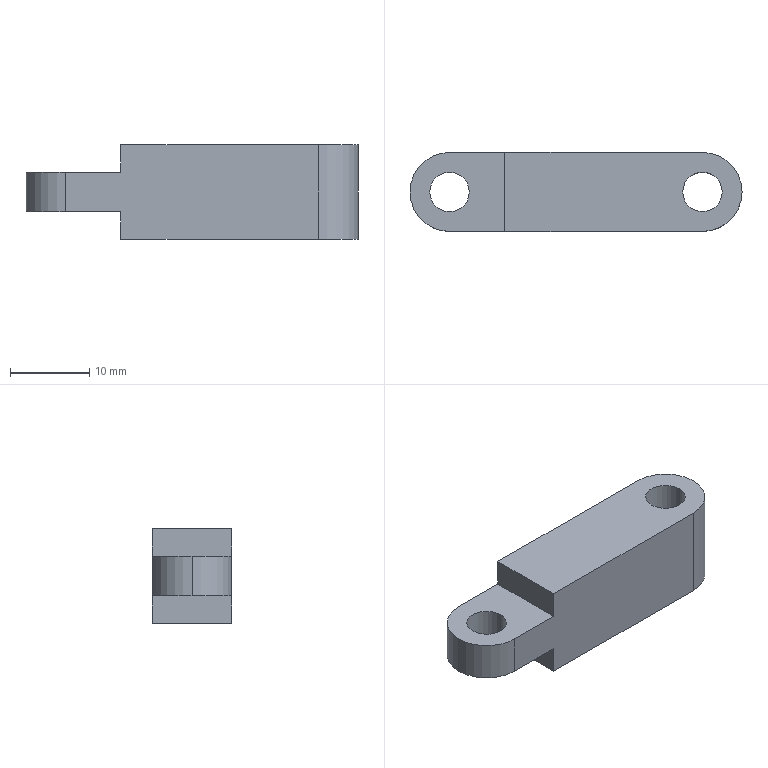Part | STEP file | gripper arm 1_default | 1 solid | 16 faces | box 42 x 10 x 12 mm | volume 3684 mm3 | cylinder 8 | plane 8 | commonest cylinder face diameters 5 x4 10 x4
STEP:
#1=CARTESIAN_POINT('',(0.,0.,0.));
#2=DIRECTION('',(0.,0.,1.));
#3=DIRECTION('',(1.,0.,0.));
#4=AXIS2_PLACEMENT_3D('',#1,#2,#3);
#5=CARTESIAN_POINT('',(18.5,0.,0.));
#6=VERTEX_POINT('',#5);
#7=CARTESIAN_POINT('',(18.5,0.,12.));
#8=VERTEX_POINT('',#7);
#9=CARTESIAN_POINT('',(18.5,0.,0.));
#10=DIRECTION('',(0.,0.,1.));
#11=VECTOR('',#10,1.);
#12=LINE('',#9,#11);
#13=CARTESIAN_POINT('',(16.,0.,0.));
#14=DIRECTION('',(0.,0.,1.));
#15=DIRECTION('',(1.,0.,0.));
#16=AXIS2_PLACEMENT_3D('',#13,#14,#15);
#17=CYLINDRICAL_SURFACE('',#16,2.5);
#18=CARTESIAN_POINT('',(6.283,0.));
#19=DIRECTION('',(0.,1.));
#20=VECTOR('',#19,1.);
#21=LINE('',#18,#20);
#22=(GEOMETRIC_REPRESENTATION_CONTEXT(2)PARAMETRIC_REPRESENTATION_CONTEXT()REPRESENTATION_CONTEXT('',''));
#23=DEFINITIONAL_REPRESENTATION('',(#21),#22);
#24=PCURVE('',#17,#23);
#25=CARTESIAN_POINT('',(16.,0.,0.));
#26=DIRECTION('',(0.,0.,1.));
#27=DIRECTION('',(1.,0.,0.));
#28=AXIS2_PLACEMENT_3D('',#25,#26,#27);
#29=CYLINDRICAL_SURFACE('',#28,2.5);
#30=CARTESIAN_POINT('',(0.,0.));
#31=DIRECTION('',(0.,1.));
#32=VECTOR('',#31,1.);
#33=LINE('',#30,#32);
#34=(GEOMETRIC_REPRESENTATION_CONTEXT(2)PARAMETRIC_REPRESENTATION_CONTEXT()REPRESENTATION_CONTEXT('',''));
#35=DEFINITIONAL_REPRESENTATION('',(#33),#34);
#36=PCURVE('',#29,#35);
#37=SURFACE_CURVE('',#12,(#24,#36),.PCURVE_S1.);
#38=EDGE_CURVE('',#6,#8,#37,.T.);
#39=ORIENTED_EDGE('',*,*,#38,.T.);
#40=CARTESIAN_POINT('',(13.5,0.,12.));
#41=VERTEX_POINT('',#40);
#42=CARTESIAN_POINT('',(16.,0.,12.));
#43=DIRECTION('',(0.,0.,1.));
#44=DIRECTION('',(1.,0.,0.));
#45=AXIS2_PLACEMENT_3D('',#42,#43,#44);
#46=CIRCLE('',#45,2.5);
#47=CARTESIAN_POINT('',(0.,12.));
#48=DIRECTION('',(1.,0.));
#49=VECTOR('',#48,1.);
#50=LINE('',#47,#49);
#51=(GEOMETRIC_REPRESENTATION_CONTEXT(2)PARAMETRIC_REPRESENTATION_CONTEXT()REPRESENTATION_CONTEXT('',''));
#52=DEFINITIONAL_REPRESENTATION('',(#50),#51);
#53=PCURVE('',#17,#52);
#54=CARTESIAN_POINT('',(0.,0.,12.));
#55=DIRECTION('',(0.,0.,1.));
#56=DIRECTION('',(1.,0.,0.));
#57=AXIS2_PLACEMENT_3D('',#54,#55,#56);
#58=PLANE('',#57);
#59=CARTESIAN_POINT('',(16.,0.));
#60=DIRECTION('',(1.,0.));
#61=AXIS2_PLACEMENT_2D('',#59,#60);
#62=CIRCLE('',#61,2.5);
#63=(GEOMETRIC_REPRESENTATION_CONTEXT(2)PARAMETRIC_REPRESENTATION_CONTEXT()REPRESENTATION_CONTEXT('',''));
#64=DEFINITIONAL_REPRESENTATION('',(#62),#63);
#65=PCURVE('',#58,#64);
#66=SURFACE_CURVE('',#46,(#53,#65),.PCURVE_S1.);
#67=EDGE_CURVE('',#41,#8,#66,.T.);
#68=ORIENTED_EDGE('',*,*,#67,.F.);
#69=CARTESIAN_POINT('',(13.5,0.,0.));
#70=VERTEX_POINT('',#69);
#71=CARTESIAN_POINT('',(13.5,0.,0.));
#72=DIRECTION('',(0.,0.,1.));
#73=VECTOR('',#72,1.);
#74=LINE('',#71,#73);
#75=CARTESIAN_POINT('',(3.142,0.));
#76=DIRECTION('',(0.,1.));
#77=VECTOR('',#76,1.);
#78=LINE('',#75,#77);
#79=(GEOMETRIC_REPRESENTATION_CONTEXT(2)PARAMETRIC_REPRESENTATION_CONTEXT()REPRESENTATION_CONTEXT('',''));
#80=DEFINITIONAL_REPRESENTATION('',(#78),#79);
#81=PCURVE('',#17,#80);
#82=CARTESIAN_POINT('',(3.142,0.));
#83=DIRECTION('',(0.,1.));
#84=VECTOR('',#83,1.);
#85=LINE('',#82,#84);
#86=(GEOMETRIC_REPRESENTATION_CONTEXT(2)PARAMETRIC_REPRESENTATION_CONTEXT()REPRESENTATION_CONTEXT('',''));
#87=DEFINITIONAL_REPRESENTATION('',(#85),#86);
#88=PCURVE('',#29,#87);
#89=SURFACE_CURVE('',#74,(#81,#88),.PCURVE_S1.);
#90=EDGE_CURVE('',#70,#41,#89,.T.);
#91=ORIENTED_EDGE('',*,*,#90,.F.);
#92=CARTESIAN_POINT('',(16.,0.,0.));
#93=DIRECTION('',(0.,0.,1.));
#94=DIRECTION('',(1.,0.,0.));
#95=AXIS2_PLACEMENT_3D('',#92,#93,#94);
#96=CIRCLE('',#95,2.5);
#97=CARTESIAN_POINT('',(0.,0.));
#98=DIRECTION('',(1.,0.));
#99=VECTOR('',#98,1.);
#100=LINE('',#97,#99);
#101=(GEOMETRIC_REPRESENTATION_CONTEXT(2)PARAMETRIC_REPRESENTATION_CONTEXT()REPRESENTATION_CONTEXT('',''));
#102=DEFINITIONAL_REPRESENTATION('',(#100),#101);
#103=PCURVE('',#17,#102);
#104=CARTESIAN_POINT('',(0.,0.,0.));
#105=DIRECTION('',(0.,0.,1.));
#106=DIRECTION('',(1.,0.,0.));
#107=AXIS2_PLACEMENT_3D('',#104,#105,#106);
#108=PLANE('',#107);
#109=CARTESIAN_POINT('',(16.,0.));
#110=DIRECTION('',(1.,0.));
#111=AXIS2_PLACEMENT_2D('',#109,#110);
#112=CIRCLE('',#111,2.5);
#113=(GEOMETRIC_REPRESENTATION_CONTEXT(2)PARAMETRIC_REPRESENTATION_CONTEXT()REPRESENTATION_CONTEXT('',''));
#114=DEFINITIONAL_REPRESENTATION('',(#112),#113);
#115=PCURVE('',#108,#114);
#116=SURFACE_CURVE('',#96,(#103,#115),.PCURVE_S1.);
#117=EDGE_CURVE('',#70,#6,#116,.T.);
#118=ORIENTED_EDGE('',*,*,#117,.T.);
#119=EDGE_LOOP('',(#39,#68,#91,#118));
#120=FACE_BOUND('',#119,.F.);
#121=ADVANCED_FACE('',(#120),#17,.F.);
#122=CARTESIAN_POINT('',(-13.5,0.,3.5));
#123=VERTEX_POINT('',#122);
#124=CARTESIAN_POINT('',(-13.5,0.,8.5));
#125=VERTEX_POINT('',#124);
#126=CARTESIAN_POINT('',(-13.5,0.,0.));
#127=DIRECTION('',(0.,0.,1.));
#128=VECTOR('',#127,1.);
#129=LINE('',#126,#128);
#130=CARTESIAN_POINT('',(-16.,0.,0.));
#131=DIRECTION('',(0.,0.,1.));
#132=DIRECTION('',(1.,0.,0.));
#133=AXIS2_PLACEMENT_3D('',#130,#131,#132);
#134=CYLINDRICAL_SURFACE('',#133,2.5);
#135=CARTESIAN_POINT('',(6.283,0.));
#136=DIRECTION('',(0.,1.));
#137=VECTOR('',#136,1.);
#138=LINE('',#135,#137);
#139=(GEOMETRIC_REPRESENTATION_CONTEXT(2)PARAMETRIC_REPRESENTATION_CONTEXT()REPRESENTATION_CONTEXT('',''));
#140=DEFINITIONAL_REPRESENTATION('',(#138),#139);
#141=PCURVE('',#134,#140);
#142=CARTESIAN_POINT('',(-16.,0.,0.));
#143=DIRECTION('',(0.,0.,1.));
#144=DIRECTION('',(1.,0.,0.));
#145=AXIS2_PLACEMENT_3D('',#142,#143,#144);
#146=CYLINDRICAL_SURFACE('',#145,2.5);
#147=CARTESIAN_POINT('',(0.,0.));
#148=DIRECTION('',(0.,1.));
#149=VECTOR('',#148,1.);
#150=LINE('',#147,#149);
#151=(GEOMETRIC_REPRESENTATION_CONTEXT(2)PARAMETRIC_REPRESENTATION_CONTEXT()REPRESENTATION_CONTEXT('',''));
#152=DEFINITIONAL_REPRESENTATION('',(#150),#151);
#153=PCURVE('',#146,#152);
#154=SURFACE_CURVE('',#129,(#141,#153),.PCURVE_S1.);
#155=EDGE_CURVE('',#123,#125,#154,.T.);
#156=ORIENTED_EDGE('',*,*,#155,.T.);
#157=CARTESIAN_POINT('',(-18.5,0.,8.5));
#158=VERTEX_POINT('',#157);
#159=CARTESIAN_POINT('',(-16.,0.,8.5));
#160=DIRECTION('',(0.,0.,-1.));
#161=DIRECTION('',(1.,0.,0.));
#162=AXIS2_PLACEMENT_3D('',#159,#160,#161);
#163=CIRCLE('',#162,2.5);
#164=CARTESIAN_POINT('',(6.283,8.5));
#165=DIRECTION('',(-1.,0.));
#166=VECTOR('',#165,1.);
#167=LINE('',#164,#166);
#168=(GEOMETRIC_REPRESENTATION_CONTEXT(2)PARAMETRIC_REPRESENTATION_CONTEXT()REPRESENTATION_CONTEXT('',''));
#169=DEFINITIONAL_REPRESENTATION('',(#167),#168);
#170=PCURVE('',#134,#169);
#171=CARTESIAN_POINT('',(0.,0.,8.5));
#172=DIRECTION('',(0.,0.,1.));
#173=DIRECTION('',(1.,0.,0.));
#174=AXIS2_PLACEMENT_3D('',#171,#172,#173);
#175=PLANE('',#174);
#176=CARTESIAN_POINT('',(-13.5,0.));
#177=CARTESIAN_POINT('',(-13.5,-4.33));
#178=CARTESIAN_POINT('',(-17.25,-2.165));
#179=CARTESIAN_POINT('',(-21.,0.));
#180=CARTESIAN_POINT('',(-17.25,2.165));
#181=CARTESIAN_POINT('',(-13.5,4.33));
#182=CARTESIAN_POINT('',(-13.5,0.));
#183=(BOUNDED_CURVE()B_SPLINE_CURVE(2,(#176,#177,#178,#179,#180,#181,#182),.UNSPECIFIED.,.T.,.F.)B_SPLINE_CURVE_WITH_KNOTS((1,2,2,2,2,1),(-2.094,0.,2.094,4.189,6.283,8.378),.UNSPECIFIED.)CURVE()GEOMETRIC_REPRESENTATION_ITEM()RATIONAL_B_SPLINE_CURVE((1.,0.5,1.,0.5,1.,0.5,1.))REPRESENTATION_ITEM(''));
#184=(GEOMETRIC_REPRESENTATION_CONTEXT(2)PARAMETRIC_REPRESENTATION_CONTEXT()REPRESENTATION_CONTEXT('',''));
#185=DEFINITIONAL_REPRESENTATION('',(#183),#184);
#186=PCURVE('',#175,#185);
#187=SURFACE_CURVE('',#163,(#170,#186),.PCURVE_S1.);
#188=EDGE_CURVE('',#125,#158,#187,.T.);
#189=ORIENTED_EDGE('',*,*,#188,.T.);
#190=CARTESIAN_POINT('',(-18.5,0.,3.5));
#191=VERTEX_POINT('',#190);
#192=CARTESIAN_POINT('',(-18.5,0.,0.));
#193=DIRECTION('',(0.,0.,1.));
#194=VECTOR('',#193,1.);
#195=LINE('',#192,#194);
#196=CARTESIAN_POINT('',(3.142,0.));
#197=DIRECTION('',(0.,1.));
#198=VECTOR('',#197,1.);
#199=LINE('',#196,#198);
#200=(GEOMETRIC_REPRESENTATION_CONTEXT(2)PARAMETRIC_REPRESENTATION_CONTEXT()REPRESENTATION_CONTEXT('',''));
#201=DEFINITIONAL_REPRESENTATION('',(#199),#200);
#202=PCURVE('',#134,#201);
#203=CARTESIAN_POINT('',(3.142,0.));
#204=DIRECTION('',(0.,1.));
#205=VECTOR('',#204,1.);
#206=LINE('',#203,#205);
#207=(GEOMETRIC_REPRESENTATION_CONTEXT(2)PARAMETRIC_REPRESENTATION_CONTEXT()REPRESENTATION_CONTEXT('',''));
#208=DEFINITIONAL_REPRESENTATION('',(#206),#207);
#209=PCURVE('',#146,#208);
#210=SURFACE_CURVE('',#195,(#202,#209),.PCURVE_S1.);
#211=EDGE_CURVE('',#191,#158,#210,.T.);
#212=ORIENTED_EDGE('',*,*,#211,.F.);
#213=CARTESIAN_POINT('',(-16.,0.,3.5));
#214=DIRECTION('',(0.,0.,1.));
#215=DIRECTION('',(-1.,0.,0.));
#216=AXIS2_PLACEMENT_3D('',#213,#214,#215);
#217=CIRCLE('',#216,2.5);
#218=CARTESIAN_POINT('',(3.142,3.5));
#219=DIRECTION('',(1.,0.));
#220=VECTOR('',#219,1.);
#221=LINE('',#218,#220);
#222=(GEOMETRIC_REPRESENTATION_CONTEXT(2)PARAMETRIC_REPRESENTATION_CONTEXT()REPRESENTATION_CONTEXT('',''));
#223=DEFINITIONAL_REPRESENTATION('',(#221),#222);
#224=PCURVE('',#134,#223);
#225=CARTESIAN_POINT('',(0.,0.,3.5));
#226=DIRECTION('',(0.,0.,-1.));
#227=DIRECTION('',(-1.,0.,0.));
#228=AXIS2_PLACEMENT_3D('',#225,#226,#227);
#229=PLANE('',#228);
#230=CARTESIAN_POINT('',(18.5,0.));
#231=CARTESIAN_POINT('',(18.5,-4.33));
#232=CARTESIAN_POINT('',(14.75,-2.165));
#233=CARTESIAN_POINT('',(11.,0.));
#234=CARTESIAN_POINT('',(14.75,2.165));
#235=CARTESIAN_POINT('',(18.5,4.33));
#236=CARTESIAN_POINT('',(18.5,0.));
#237=(BOUNDED_CURVE()B_SPLINE_CURVE(2,(#230,#231,#232,#233,#234,#235,#236),.UNSPECIFIED.,.T.,.F.)B_SPLINE_CURVE_WITH_KNOTS((1,2,2,2,2,1),(-2.094,0.,2.094,4.189,6.283,8.378),.UNSPECIFIED.)CURVE()GEOMETRIC_REPRESENTATION_ITEM()RATIONAL_B_SPLINE_CURVE((1.,0.5,1.,0.5,1.,0.5,1.))REPRESENTATION_ITEM(''));
#238=(GEOMETRIC_REPRESENTATION_CONTEXT(2)PARAMETRIC_REPRESENTATION_CONTEXT()REPRESENTATION_CONTEXT('',''));
#239=DEFINITIONAL_REPRESENTATION('',(#237),#238);
#240=PCURVE('',#229,#239);
#241=SURFACE_CURVE('',#217,(#224,#240),.PCURVE_S1.);
#242=EDGE_CURVE('',#191,#123,#241,.T.);
#243=ORIENTED_EDGE('',*,*,#242,.T.);
#244=EDGE_LOOP('',(#156,#189,#212,#243));
#245=FACE_BOUND('',#244,.F.);
#246=ADVANCED_FACE('',(#245),#134,.F.);
#247=CARTESIAN_POINT('',(-16.,0.,8.5));
#248=DIRECTION('',(0.,0.,-1.));
#249=DIRECTION('',(1.,0.,0.));
#250=AXIS2_PLACEMENT_3D('',#247,#248,#249);
#251=CIRCLE('',#250,2.5);
#252=CARTESIAN_POINT('',(6.283,8.5));
#253=DIRECTION('',(-1.,0.));
#254=VECTOR('',#253,1.);
#255=LINE('',#252,#254);
#256=(GEOMETRIC_REPRESENTATION_CONTEXT(2)PARAMETRIC_REPRESENTATION_CONTEXT()REPRESENTATION_CONTEXT('',''));
#257=DEFINITIONAL_REPRESENTATION('',(#255),#256);
#258=PCURVE('',#146,#257);
#259=CARTESIAN_POINT('',(-13.5,0.));
#260=CARTESIAN_POINT('',(-13.5,-4.33));
#261=CARTESIAN_POINT('',(-17.25,-2.165));
#262=CARTESIAN_POINT('',(-21.,0.));
#263=CARTESIAN_POINT('',(-17.25,2.165));
#264=CARTESIAN_POINT('',(-13.5,4.33));
#265=CARTESIAN_POINT('',(-13.5,0.));
#266=(BOUNDED_CURVE()B_SPLINE_CURVE(2,(#259,#260,#261,#262,#263,#264,#265),.UNSPECIFIED.,.T.,.F.)B_SPLINE_CURVE_WITH_KNOTS((1,2,2,2,2,1),(-2.094,0.,2.094,4.189,6.283,8.378),.UNSPECIFIED.)CURVE()GEOMETRIC_REPRESENTATION_ITEM()RATIONAL_B_SPLINE_CURVE((1.,0.5,1.,0.5,1.,0.5,1.))REPRESENTATION_ITEM(''));
#267=(GEOMETRIC_REPRESENTATION_CONTEXT(2)PARAMETRIC_REPRESENTATION_CONTEXT()REPRESENTATION_CONTEXT('',''));
#268=DEFINITIONAL_REPRESENTATION('',(#266),#267);
#269=PCURVE('',#175,#268);
#270=SURFACE_CURVE('',#251,(#258,#269),.PCURVE_S1.);
#271=EDGE_CURVE('',#158,#125,#270,.T.);
#272=ORIENTED_EDGE('',*,*,#271,.T.);
#273=ORIENTED_EDGE('',*,*,#155,.F.);
#274=CARTESIAN_POINT('',(-16.,0.,3.5));
#275=DIRECTION('',(0.,0.,1.));
#276=DIRECTION('',(-1.,0.,0.));
#277=AXIS2_PLACEMENT_3D('',#274,#275,#276);
#278=CIRCLE('',#277,2.5);
#279=CARTESIAN_POINT('',(-3.142,3.5));
#280=DIRECTION('',(1.,0.));
#281=VECTOR('',#280,1.);
#282=LINE('',#279,#281);
#283=(GEOMETRIC_REPRESENTATION_CONTEXT(2)PARAMETRIC_REPRESENTATION_CONTEXT()REPRESENTATION_CONTEXT('',''));
#284=DEFINITIONAL_REPRESENTATION('',(#282),#283);
#285=PCURVE('',#146,#284);
#286=CARTESIAN_POINT('',(18.5,0.));
#287=CARTESIAN_POINT('',(18.5,-4.33));
#288=CARTESIAN_POINT('',(14.75,-2.165));
#289=CARTESIAN_POINT('',(11.,0.));
#290=CARTESIAN_POINT('',(14.75,2.165));
#291=CARTESIAN_POINT('',(18.5,4.33));
#292=CARTESIAN_POINT('',(18.5,0.));
#293=(BOUNDED_CURVE()B_SPLINE_CURVE(2,(#286,#287,#288,#289,#290,#291,#292),.UNSPECIFIED.,.T.,.F.)B_SPLINE_CURVE_WITH_KNOTS((1,2,2,2,2,1),(-2.094,0.,2.094,4.189,6.283,8.378),.UNSPECIFIED.)CURVE()GEOMETRIC_REPRESENTATION_ITEM()RATIONAL_B_SPLINE_CURVE((1.,0.5,1.,0.5,1.,0.5,1.))REPRESENTATION_ITEM(''));
#294=(GEOMETRIC_REPRESENTATION_CONTEXT(2)PARAMETRIC_REPRESENTATION_CONTEXT()REPRESENTATION_CONTEXT('',''));
#295=DEFINITIONAL_REPRESENTATION('',(#293),#294);
#296=PCURVE('',#229,#295);
#297=SURFACE_CURVE('',#278,(#285,#296),.PCURVE_S1.);
#298=EDGE_CURVE('',#123,#191,#297,.T.);
#299=ORIENTED_EDGE('',*,*,#298,.T.);
#300=ORIENTED_EDGE('',*,*,#211,.T.);
#301=EDGE_LOOP('',(#272,#273,#299,#300));
#302=FACE_BOUND('',#301,.F.);
#303=ADVANCED_FACE('',(#302),#146,.F.);
#304=CARTESIAN_POINT('',(-16.,5.,3.5));
#305=VERTEX_POINT('',#304);
#306=CARTESIAN_POINT('',(-16.,5.,8.5));
#307=VERTEX_POINT('',#306);
#308=CARTESIAN_POINT('',(-16.,5.,12.));
#309=DIRECTION('',(0.,0.,1.));
#310=VECTOR('',#309,1.);
#311=LINE('',#308,#310);
#312=CARTESIAN_POINT('',(-16.,0.,12.));
#313=DIRECTION('',(0.,0.,-1.));
#314=DIRECTION('',(-1.,0.,0.));
#315=AXIS2_PLACEMENT_3D('',#312,#313,#314);
#316=CYLINDRICAL_SURFACE('',#315,5.);
#317=CARTESIAN_POINT('',(1.571,0.));
#318=DIRECTION('',(0.,-1.));
#319=VECTOR('',#318,1.);
#320=LINE('',#317,#319);
#321=(GEOMETRIC_REPRESENTATION_CONTEXT(2)PARAMETRIC_REPRESENTATION_CONTEXT()REPRESENTATION_CONTEXT('',''));
#322=DEFINITIONAL_REPRESENTATION('',(#320),#321);
#323=PCURVE('',#316,#322);
#324=CARTESIAN_POINT('',(-21.,5.,12.));
#325=DIRECTION('',(0.,-1.,0.));
#326=DIRECTION('',(0.,0.,-1.));
#327=AXIS2_PLACEMENT_3D('',#324,#325,#326);
#328=PLANE('',#327);
#329=CARTESIAN_POINT('',(0.,5.));
#330=DIRECTION('',(-1.,0.));
#331=VECTOR('',#330,1.);
#332=LINE('',#329,#331);
#333=(GEOMETRIC_REPRESENTATION_CONTEXT(2)PARAMETRIC_REPRESENTATION_CONTEXT()REPRESENTATION_CONTEXT('',''));
#334=DEFINITIONAL_REPRESENTATION('',(#332),#333);
#335=PCURVE('',#328,#334);
#336=SURFACE_CURVE('',#311,(#323,#335),.PCURVE_S1.);
#337=EDGE_CURVE('',#305,#307,#336,.T.);
#338=ORIENTED_EDGE('',*,*,#337,.F.);
#339=CARTESIAN_POINT('',(-21.,0.,3.5));
#340=VERTEX_POINT('',#339);
#341=CARTESIAN_POINT('',(-16.,0.,3.5));
#342=DIRECTION('',(0.,0.,1.));
#343=DIRECTION('',(-1.,0.,0.));
#344=AXIS2_PLACEMENT_3D('',#341,#342,#343);
#345=CIRCLE('',#344,5.);
#346=CARTESIAN_POINT('',(6.283,8.5));
#347=DIRECTION('',(-1.,0.));
#348=VECTOR('',#347,1.);
#349=LINE('',#346,#348);
#350=(GEOMETRIC_REPRESENTATION_CONTEXT(2)PARAMETRIC_REPRESENTATION_CONTEXT()REPRESENTATION_CONTEXT('',''));
#351=DEFINITIONAL_REPRESENTATION('',(#349),#350);
#352=PCURVE('',#316,#351);
#353=CARTESIAN_POINT('',(21.,0.));
#354=CARTESIAN_POINT('',(21.,-8.66));
#355=CARTESIAN_POINT('',(13.5,-4.33));
#356=CARTESIAN_POINT('',(6.,0.));
#357=CARTESIAN_POINT('',(13.5,4.33));
#358=CARTESIAN_POINT('',(21.,8.66));
#359=CARTESIAN_POINT('',(21.,0.));
#360=(BOUNDED_CURVE()B_SPLINE_CURVE(2,(#353,#354,#355,#356,#357,#358,#359),.UNSPECIFIED.,.T.,.F.)B_SPLINE_CURVE_WITH_KNOTS((1,2,2,2,2,1),(-2.094,0.,2.094,4.189,6.283,8.378),.UNSPECIFIED.)CURVE()GEOMETRIC_REPRESENTATION_ITEM()RATIONAL_B_SPLINE_CURVE((1.,0.5,1.,0.5,1.,0.5,1.))REPRESENTATION_ITEM(''));
#361=(GEOMETRIC_REPRESENTATION_CONTEXT(2)PARAMETRIC_REPRESENTATION_CONTEXT()REPRESENTATION_CONTEXT('',''));
#362=DEFINITIONAL_REPRESENTATION('',(#360),#361);
#363=PCURVE('',#229,#362);
#364=SURFACE_CURVE('',#345,(#352,#363),.PCURVE_S1.);
#365=EDGE_CURVE('',#305,#340,#364,.T.);
#366=ORIENTED_EDGE('',*,*,#365,.T.);
#367=CARTESIAN_POINT('',(-21.,0.,8.5));
#368=VERTEX_POINT('',#367);
#369=CARTESIAN_POINT('',(-21.,0.,12.));
#370=DIRECTION('',(0.,0.,-1.));
#371=VECTOR('',#370,1.);
#372=LINE('',#369,#371);
#373=CARTESIAN_POINT('',(0.,0.));
#374=DIRECTION('',(0.,1.));
#375=VECTOR('',#374,1.);
#376=LINE('',#373,#375);
#377=(GEOMETRIC_REPRESENTATION_CONTEXT(2)PARAMETRIC_REPRESENTATION_CONTEXT()REPRESENTATION_CONTEXT('',''));
#378=DEFINITIONAL_REPRESENTATION('',(#376),#377);
#379=PCURVE('',#316,#378);
#380=CARTESIAN_POINT('',(-16.,0.,12.));
#381=DIRECTION('',(0.,0.,-1.));
#382=DIRECTION('',(-1.,0.,0.));
#383=AXIS2_PLACEMENT_3D('',#380,#381,#382);
#384=CYLINDRICAL_SURFACE('',#383,5.);
#385=CARTESIAN_POINT('',(6.283,0.));
#386=DIRECTION('',(0.,1.));
#387=VECTOR('',#386,1.);
#388=LINE('',#385,#387);
#389=(GEOMETRIC_REPRESENTATION_CONTEXT(2)PARAMETRIC_REPRESENTATION_CONTEXT()REPRESENTATION_CONTEXT('',''));
#390=DEFINITIONAL_REPRESENTATION('',(#388),#389);
#391=PCURVE('',#384,#390);
#392=SURFACE_CURVE('',#372,(#379,#391),.PCURVE_S1.);
#393=EDGE_CURVE('',#368,#340,#392,.T.);
#394=ORIENTED_EDGE('',*,*,#393,.F.);
#395=CARTESIAN_POINT('',(-16.,0.,8.5));
#396=DIRECTION('',(0.,0.,-1.));
#397=DIRECTION('',(1.,0.,0.));
#398=AXIS2_PLACEMENT_3D('',#395,#396,#397);
#399=CIRCLE('',#398,5.);
#400=CARTESIAN_POINT('',(-3.142,3.5));
#401=DIRECTION('',(1.,0.));
#402=VECTOR('',#401,1.);
#403=LINE('',#400,#402);
#404=(GEOMETRIC_REPRESENTATION_CONTEXT(2)PARAMETRIC_REPRESENTATION_CONTEXT()REPRESENTATION_CONTEXT('',''));
#405=DEFINITIONAL_REPRESENTATION('',(#403),#404);
#406=PCURVE('',#316,#405);
#407=CARTESIAN_POINT('',(-11.,0.));
#408=CARTESIAN_POINT('',(-11.,-8.66));
#409=CARTESIAN_POINT('',(-18.5,-4.33));
#410=CARTESIAN_POINT('',(-26.,0.));
#411=CARTESIAN_POINT('',(-18.5,4.33));
#412=CARTESIAN_POINT('',(-11.,8.66));
#413=CARTESIAN_POINT('',(-11.,0.));
#414=(BOUNDED_CURVE()B_SPLINE_CURVE(2,(#407,#408,#409,#410,#411,#412,#413),.UNSPECIFIED.,.T.,.F.)B_SPLINE_CURVE_WITH_KNOTS((1,2,2,2,2,1),(-2.094,0.,2.094,4.189,6.283,8.378),.UNSPECIFIED.)CURVE()GEOMETRIC_REPRESENTATION_ITEM()RATIONAL_B_SPLINE_CURVE((1.,0.5,1.,0.5,1.,0.5,1.))REPRESENTATION_ITEM(''));
#415=(GEOMETRIC_REPRESENTATION_CONTEXT(2)PARAMETRIC_REPRESENTATION_CONTEXT()REPRESENTATION_CONTEXT('',''));
#416=DEFINITIONAL_REPRESENTATION('',(#414),#415);
#417=PCURVE('',#175,#416);
#418=SURFACE_CURVE('',#399,(#406,#417),.PCURVE_S1.);
#419=EDGE_CURVE('',#368,#307,#418,.T.);
#420=ORIENTED_EDGE('',*,*,#419,.T.);
#421=EDGE_LOOP('',(#338,#366,#394,#420));
#422=FACE_BOUND('',#421,.T.);
#423=ADVANCED_FACE('',(#422),#316,.T.);
#424=ORIENTED_EDGE('',*,*,#393,.T.);
#425=CARTESIAN_POINT('',(-16.,-5.,3.5));
#426=VERTEX_POINT('',#425);
#427=CARTESIAN_POINT('',(-16.,0.,3.5));
#428=DIRECTION('',(0.,0.,1.));
#429=DIRECTION('',(-1.,0.,0.));
#430=AXIS2_PLACEMENT_3D('',#427,#428,#429);
#431=CIRCLE('',#430,5.);
#432=CARTESIAN_POINT('',(6.283,8.5));
#433=DIRECTION('',(-1.,0.));
#434=VECTOR('',#433,1.);
#435=LINE('',#432,#434);
#436=(GEOMETRIC_REPRESENTATION_CONTEXT(2)PARAMETRIC_REPRESENTATION_CONTEXT()REPRESENTATION_CONTEXT('',''));
#437=DEFINITIONAL_REPRESENTATION('',(#435),#436);
#438=PCURVE('',#384,#437);
#439=CARTESIAN_POINT('',(21.,0.));
#440=CARTESIAN_POINT('',(21.,-8.66));
#441=CARTESIAN_POINT('',(13.5,-4.33));
#442=CARTESIAN_POINT('',(6.,0.));
#443=CARTESIAN_POINT('',(13.5,4.33));
#444=CARTESIAN_POINT('',(21.,8.66));
#445=CARTESIAN_POINT('',(21.,0.));
#446=(BOUNDED_CURVE()B_SPLINE_CURVE(2,(#439,#440,#441,#442,#443,#444,#445),.UNSPECIFIED.,.T.,.F.)B_SPLINE_CURVE_WITH_KNOTS((1,2,2,2,2,1),(-2.094,0.,2.094,4.189,6.283,8.378),.UNSPECIFIED.)CURVE()GEOMETRIC_REPRESENTATION_ITEM()RATIONAL_B_SPLINE_CURVE((1.,0.5,1.,0.5,1.,0.5,1.))REPRESENTATION_ITEM(''));
#447=(GEOMETRIC_REPRESENTATION_CONTEXT(2)PARAMETRIC_REPRESENTATION_CONTEXT()REPRESENTATION_CONTEXT('',''));
#448=DEFINITIONAL_REPRESENTATION('',(#446),#447);
#449=PCURVE('',#229,#448);
#450=SURFACE_CURVE('',#431,(#438,#449),.PCURVE_S1.);
#451=EDGE_CURVE('',#340,#426,#450,.T.);
#452=ORIENTED_EDGE('',*,*,#451,.T.);
#453=CARTESIAN_POINT('',(-16.,-5.,8.5));
#454=VERTEX_POINT('',#453);
#455=CARTESIAN_POINT('',(-16.,-5.,12.));
#456=DIRECTION('',(0.,0.,-1.));
#457=VECTOR('',#456,1.);
#458=LINE('',#455,#457);
#459=CARTESIAN_POINT('',(4.712,0.));
#460=DIRECTION('',(0.,1.));
#461=VECTOR('',#460,1.);
#462=LINE('',#459,#461);
#463=(GEOMETRIC_REPRESENTATION_CONTEXT(2)PARAMETRIC_REPRESENTATION_CONTEXT()REPRESENTATION_CONTEXT('',''));
#464=DEFINITIONAL_REPRESENTATION('',(#462),#463);
#465=PCURVE('',#384,#464);
#466=CARTESIAN_POINT('',(-21.,-5.,12.));
#467=DIRECTION('',(0.,1.,0.));
#468=DIRECTION('',(0.,0.,1.));
#469=AXIS2_PLACEMENT_3D('',#466,#467,#468);
#470=PLANE('',#469);
#471=CARTESIAN_POINT('',(0.,5.));
#472=DIRECTION('',(-1.,0.));
#473=VECTOR('',#472,1.);
#474=LINE('',#471,#473);
#475=(GEOMETRIC_REPRESENTATION_CONTEXT(2)PARAMETRIC_REPRESENTATION_CONTEXT()REPRESENTATION_CONTEXT('',''));
#476=DEFINITIONAL_REPRESENTATION('',(#474),#475);
#477=PCURVE('',#470,#476);
#478=SURFACE_CURVE('',#458,(#465,#477),.PCURVE_S1.);
#479=EDGE_CURVE('',#454,#426,#478,.T.);
#480=ORIENTED_EDGE('',*,*,#479,.F.);
#481=CARTESIAN_POINT('',(-16.,0.,8.5));
#482=DIRECTION('',(0.,0.,-1.));
#483=DIRECTION('',(1.,0.,0.));
#484=AXIS2_PLACEMENT_3D('',#481,#482,#483);
#485=CIRCLE('',#484,5.);
#486=CARTESIAN_POINT('',(3.142,3.5));
#487=DIRECTION('',(1.,0.));
#488=VECTOR('',#487,1.);
#489=LINE('',#486,#488);
#490=(GEOMETRIC_REPRESENTATION_CONTEXT(2)PARAMETRIC_REPRESENTATION_CONTEXT()REPRESENTATION_CONTEXT('',''));
#491=DEFINITIONAL_REPRESENTATION('',(#489),#490);
#492=PCURVE('',#384,#491);
#493=CARTESIAN_POINT('',(-11.,0.));
#494=CARTESIAN_POINT('',(-11.,-8.66));
#495=CARTESIAN_POINT('',(-18.5,-4.33));
#496=CARTESIAN_POINT('',(-26.,0.));
#497=CARTESIAN_POINT('',(-18.5,4.33));
#498=CARTESIAN_POINT('',(-11.,8.66));
#499=CARTESIAN_POINT('',(-11.,0.));
#500=(BOUNDED_CURVE()B_SPLINE_CURVE(2,(#493,#494,#495,#496,#497,#498,#499),.UNSPECIFIED.,.T.,.F.)B_SPLINE_CURVE_WITH_KNOTS((1,2,2,2,2,1),(-2.094,0.,2.094,4.189,6.283,8.378),.UNSPECIFIED.)CURVE()GEOMETRIC_REPRESENTATION_ITEM()RATIONAL_B_SPLINE_CURVE((1.,0.5,1.,0.5,1.,0.5,1.))REPRESENTATION_ITEM(''));
#501=(GEOMETRIC_REPRESENTATION_CONTEXT(2)PARAMETRIC_REPRESENTATION_CONTEXT()REPRESENTATION_CONTEXT('',''));
#502=DEFINITIONAL_REPRESENTATION('',(#500),#501);
#503=PCURVE('',#175,#502);
#504=SURFACE_CURVE('',#485,(#492,#503),.PCURVE_S1.);
#505=EDGE_CURVE('',#454,#368,#504,.T.);
#506=ORIENTED_EDGE('',*,*,#505,.T.);
#507=EDGE_LOOP('',(#424,#452,#480,#506));
#508=FACE_BOUND('',#507,.T.);
#509=ADVANCED_FACE('',(#508),#384,.T.);
#510=CARTESIAN_POINT('',(16.,5.,0.));
#511=VERTEX_POINT('',#510);
#512=CARTESIAN_POINT('',(-9.,5.,0.));
#513=VERTEX_POINT('',#512);
#514=CARTESIAN_POINT('',(-21.,5.,0.));
#515=DIRECTION('',(-1.,0.,0.));
#516=VECTOR('',#515,1.);
#517=LINE('',#514,#516);
#518=CARTESIAN_POINT('',(12.,0.));
#519=DIRECTION('',(0.,-1.));
#520=VECTOR('',#519,1.);
#521=LINE('',#518,#520);
#522=(GEOMETRIC_REPRESENTATION_CONTEXT(2)PARAMETRIC_REPRESENTATION_CONTEXT()REPRESENTATION_CONTEXT('',''));
#523=DEFINITIONAL_REPRESENTATION('',(#521),#522);
#524=PCURVE('',#328,#523);
#525=CARTESIAN_POINT('',(-21.,5.));
#526=DIRECTION('',(-1.,0.));
#527=VECTOR('',#526,1.);
#528=LINE('',#525,#527);
#529=(GEOMETRIC_REPRESENTATION_CONTEXT(2)PARAMETRIC_REPRESENTATION_CONTEXT()REPRESENTATION_CONTEXT('',''));
#530=DEFINITIONAL_REPRESENTATION('',(#528),#529);
#531=PCURVE('',#108,#530);
#532=SURFACE_CURVE('',#517,(#524,#531),.PCURVE_S1.);
#533=EDGE_CURVE('',#511,#513,#532,.T.);
#534=ORIENTED_EDGE('',*,*,#533,.T.);
#535=CARTESIAN_POINT('',(-9.,5.,3.5));
#536=VERTEX_POINT('',#535);
#537=CARTESIAN_POINT('',(-9.,5.,12.));
#538=DIRECTION('',(0.,0.,1.));
#539=VECTOR('',#538,1.);
#540=LINE('',#537,#539);
#541=CARTESIAN_POINT('',(0.,12.));
#542=DIRECTION('',(-1.,0.));
#543=VECTOR('',#542,1.);
#544=LINE('',#541,#543);
#545=(GEOMETRIC_REPRESENTATION_CONTEXT(2)PARAMETRIC_REPRESENTATION_CONTEXT()REPRESENTATION_CONTEXT('',''));
#546=DEFINITIONAL_REPRESENTATION('',(#544),#545);
#547=PCURVE('',#328,#546);
#548=CARTESIAN_POINT('',(-9.,6.326,3.5));
#549=DIRECTION('',(1.,0.,0.));
#550=DIRECTION('',(0.,1.,0.));
#551=AXIS2_PLACEMENT_3D('',#548,#549,#550);
#552=PLANE('',#551);
#553=CARTESIAN_POINT('',(-1.326,8.5));
#554=DIRECTION('',(0.,1.));
#555=VECTOR('',#554,1.);
#556=LINE('',#553,#555);
#557=(GEOMETRIC_REPRESENTATION_CONTEXT(2)PARAMETRIC_REPRESENTATION_CONTEXT()REPRESENTATION_CONTEXT('',''));
#558=DEFINITIONAL_REPRESENTATION('',(#556),#557);
#559=PCURVE('',#552,#558);
#560=SURFACE_CURVE('',#540,(#547,#559),.PCURVE_S1.);
#561=EDGE_CURVE('',#513,#536,#560,.T.);
#562=ORIENTED_EDGE('',*,*,#561,.T.);
#563=CARTESIAN_POINT('',(-21.,5.,3.5));
#564=DIRECTION('',(1.,0.,0.));
#565=VECTOR('',#564,1.);
#566=LINE('',#563,#565);
#567=CARTESIAN_POINT('',(8.5,0.));
#568=DIRECTION('',(0.,1.));
#569=VECTOR('',#568,1.);
#570=LINE('',#567,#569);
#571=(GEOMETRIC_REPRESENTATION_CONTEXT(2)PARAMETRIC_REPRESENTATION_CONTEXT()REPRESENTATION_CONTEXT('',''));
#572=DEFINITIONAL_REPRESENTATION('',(#570),#571);
#573=PCURVE('',#328,#572);
#574=CARTESIAN_POINT('',(21.,5.));
#575=DIRECTION('',(-1.,0.));
#576=VECTOR('',#575,1.);
#577=LINE('',#574,#576);
#578=(GEOMETRIC_REPRESENTATION_CONTEXT(2)PARAMETRIC_REPRESENTATION_CONTEXT()REPRESENTATION_CONTEXT('',''));
#579=DEFINITIONAL_REPRESENTATION('',(#577),#578);
#580=PCURVE('',#229,#579);
#581=SURFACE_CURVE('',#566,(#573,#580),.PCURVE_S1.);
#582=EDGE_CURVE('',#305,#536,#581,.T.);
#583=ORIENTED_EDGE('',*,*,#582,.F.);
#584=ORIENTED_EDGE('',*,*,#337,.T.);
#585=CARTESIAN_POINT('',(-9.,5.,8.5));
#586=VERTEX_POINT('',#585);
#587=CARTESIAN_POINT('',(-21.,5.,8.5));
#588=DIRECTION('',(-1.,0.,0.));
#589=VECTOR('',#588,1.);
#590=LINE('',#587,#589);
#591=CARTESIAN_POINT('',(3.5,0.));
#592=DIRECTION('',(0.,-1.));
#593=VECTOR('',#592,1.);
#594=LINE('',#591,#593);
#595=(GEOMETRIC_REPRESENTATION_CONTEXT(2)PARAMETRIC_REPRESENTATION_CONTEXT()REPRESENTATION_CONTEXT('',''));
#596=DEFINITIONAL_REPRESENTATION('',(#594),#595);
#597=PCURVE('',#328,#596);
#598=CARTESIAN_POINT('',(-21.,5.));
#599=DIRECTION('',(-1.,0.));
#600=VECTOR('',#599,1.);
#601=LINE('',#598,#600);
#602=(GEOMETRIC_REPRESENTATION_CONTEXT(2)PARAMETRIC_REPRESENTATION_CONTEXT()REPRESENTATION_CONTEXT('',''));
#603=DEFINITIONAL_REPRESENTATION('',(#601),#602);
#604=PCURVE('',#175,#603);
#605=SURFACE_CURVE('',#590,(#597,#604),.PCURVE_S1.);
#606=EDGE_CURVE('',#586,#307,#605,.T.);
#607=ORIENTED_EDGE('',*,*,#606,.F.);
#608=CARTESIAN_POINT('',(-9.,5.,12.));
#609=VERTEX_POINT('',#608);
#610=CARTESIAN_POINT('',(-9.,5.,12.));
#611=DIRECTION('',(0.,0.,1.));
#612=VECTOR('',#611,1.);
#613=LINE('',#610,#612);
#614=CARTESIAN_POINT('',(0.,12.));
#615=DIRECTION('',(-1.,0.));
#616=VECTOR('',#615,1.);
#617=LINE('',#614,#616);
#618=(GEOMETRIC_REPRESENTATION_CONTEXT(2)PARAMETRIC_REPRESENTATION_CONTEXT()REPRESENTATION_CONTEXT('',''));
#619=DEFINITIONAL_REPRESENTATION('',(#617),#618);
#620=PCURVE('',#328,#619);
#621=CARTESIAN_POINT('',(-9.,7.188,8.5));
#622=DIRECTION('',(1.,0.,0.));
#623=DIRECTION('',(0.,0.,-1.));
#624=AXIS2_PLACEMENT_3D('',#621,#622,#623);
#625=PLANE('',#624);
#626=CARTESIAN_POINT('',(-3.5,-2.188));
#627=DIRECTION('',(-1.,0.));
#628=VECTOR('',#627,1.);
#629=LINE('',#626,#628);
#630=(GEOMETRIC_REPRESENTATION_CONTEXT(2)PARAMETRIC_REPRESENTATION_CONTEXT()REPRESENTATION_CONTEXT('',''));
#631=DEFINITIONAL_REPRESENTATION('',(#629),#630);
#632=PCURVE('',#625,#631);
#633=SURFACE_CURVE('',#613,(#620,#632),.PCURVE_S1.);
#634=EDGE_CURVE('',#586,#609,#633,.T.);
#635=ORIENTED_EDGE('',*,*,#634,.T.);
#636=CARTESIAN_POINT('',(16.,5.,12.));
#637=VERTEX_POINT('',#636);
#638=CARTESIAN_POINT('',(-21.,5.,12.));
#639=DIRECTION('',(-1.,0.,0.));
#640=VECTOR('',#639,1.);
#641=LINE('',#638,#640);
#642=CARTESIAN_POINT('',(0.,0.));
#643=DIRECTION('',(0.,-1.));
#644=VECTOR('',#643,1.);
#645=LINE('',#642,#644);
#646=(GEOMETRIC_REPRESENTATION_CONTEXT(2)PARAMETRIC_REPRESENTATION_CONTEXT()REPRESENTATION_CONTEXT('',''));
#647=DEFINITIONAL_REPRESENTATION('',(#645),#646);
#648=PCURVE('',#328,#647);
#649=CARTESIAN_POINT('',(-21.,5.));
#650=DIRECTION('',(-1.,0.));
#651=VECTOR('',#650,1.);
#652=LINE('',#649,#651);
#653=(GEOMETRIC_REPRESENTATION_CONTEXT(2)PARAMETRIC_REPRESENTATION_CONTEXT()REPRESENTATION_CONTEXT('',''));
#654=DEFINITIONAL_REPRESENTATION('',(#652),#653);
#655=PCURVE('',#58,#654);
#656=SURFACE_CURVE('',#641,(#648,#655),.PCURVE_S1.);
#657=EDGE_CURVE('',#637,#609,#656,.T.);
#658=ORIENTED_EDGE('',*,*,#657,.F.);
#659=CARTESIAN_POINT('',(16.,5.,12.));
#660=DIRECTION('',(0.,0.,-1.));
#661=VECTOR('',#660,1.);
#662=LINE('',#659,#661);
#663=CARTESIAN_POINT('',(0.,37.));
#664=DIRECTION('',(1.,0.));
#665=VECTOR('',#664,1.);
#666=LINE('',#663,#665);
#667=(GEOMETRIC_REPRESENTATION_CONTEXT(2)PARAMETRIC_REPRESENTATION_CONTEXT()REPRESENTATION_CONTEXT('',''));
#668=DEFINITIONAL_REPRESENTATION('',(#666),#667);
#669=PCURVE('',#328,#668);
#670=CARTESIAN_POINT('',(16.,0.,12.));
#671=DIRECTION('',(0.,0.,-1.));
#672=DIRECTION('',(-1.,0.,0.));
#673=AXIS2_PLACEMENT_3D('',#670,#671,#672);
#674=CYLINDRICAL_SURFACE('',#673,5.);
#675=CARTESIAN_POINT('',(1.571,0.));
#676=DIRECTION('',(0.,1.));
#677=VECTOR('',#676,1.);
#678=LINE('',#675,#677);
#679=(GEOMETRIC_REPRESENTATION_CONTEXT(2)PARAMETRIC_REPRESENTATION_CONTEXT()REPRESENTATION_CONTEXT('',''));
#680=DEFINITIONAL_REPRESENTATION('',(#678),#679);
#681=PCURVE('',#674,#680);
#682=SURFACE_CURVE('',#662,(#669,#681),.PCURVE_S1.);
#683=EDGE_CURVE('',#637,#511,#682,.T.);
#684=ORIENTED_EDGE('',*,*,#683,.T.);
#685=EDGE_LOOP('',(#534,#562,#583,#584,#607,#635,#658,#684));
#686=FACE_BOUND('',#685,.T.);
#687=ADVANCED_FACE('',(#686),#328,.F.);
#688=CARTESIAN_POINT('',(-9.,-5.,3.5));
#689=VERTEX_POINT('',#688);
#690=CARTESIAN_POINT('',(-21.,-5.,3.5));
#691=DIRECTION('',(-1.,0.,0.));
#692=VECTOR('',#691,1.);
#693=LINE('',#690,#692);
#694=CARTESIAN_POINT('',(-8.5,0.));
#695=DIRECTION('',(0.,-1.));
#696=VECTOR('',#695,1.);
#697=LINE('',#694,#696);
#698=(GEOMETRIC_REPRESENTATION_CONTEXT(2)PARAMETRIC_REPRESENTATION_CONTEXT()REPRESENTATION_CONTEXT('',''));
#699=DEFINITIONAL_REPRESENTATION('',(#697),#698);
#700=PCURVE('',#470,#699);
#701=CARTESIAN_POINT('',(21.,-5.));
#702=DIRECTION('',(1.,0.));
#703=VECTOR('',#702,1.);
#704=LINE('',#701,#703);
#705=(GEOMETRIC_REPRESENTATION_CONTEXT(2)PARAMETRIC_REPRESENTATION_CONTEXT()REPRESENTATION_CONTEXT('',''));
#706=DEFINITIONAL_REPRESENTATION('',(#704),#705);
#707=PCURVE('',#229,#706);
#708=SURFACE_CURVE('',#693,(#700,#707),.PCURVE_S1.);
#709=EDGE_CURVE('',#689,#426,#708,.T.);
#710=ORIENTED_EDGE('',*,*,#709,.F.);
#711=CARTESIAN_POINT('',(-9.,-5.,0.));
#712=VERTEX_POINT('',#711);
#713=CARTESIAN_POINT('',(-9.,-5.,12.));
#714=DIRECTION('',(0.,0.,-1.));
#715=VECTOR('',#714,1.);
#716=LINE('',#713,#715);
#717=CARTESIAN_POINT('',(0.,12.));
#718=DIRECTION('',(-1.,0.));
#719=VECTOR('',#718,1.);
#720=LINE('',#717,#719);
#721=(GEOMETRIC_REPRESENTATION_CONTEXT(2)PARAMETRIC_REPRESENTATION_CONTEXT()REPRESENTATION_CONTEXT('',''));
#722=DEFINITIONAL_REPRESENTATION('',(#720),#721);
#723=PCURVE('',#470,#722);
#724=CARTESIAN_POINT('',(-11.326,8.5));
#725=DIRECTION('',(0.,-1.));
#726=VECTOR('',#725,1.);
#727=LINE('',#724,#726);
#728=(GEOMETRIC_REPRESENTATION_CONTEXT(2)PARAMETRIC_REPRESENTATION_CONTEXT()REPRESENTATION_CONTEXT('',''));
#729=DEFINITIONAL_REPRESENTATION('',(#727),#728);
#730=PCURVE('',#552,#729);
#731=SURFACE_CURVE('',#716,(#723,#730),.PCURVE_S1.);
#732=EDGE_CURVE('',#689,#712,#731,.T.);
#733=ORIENTED_EDGE('',*,*,#732,.T.);
#734=CARTESIAN_POINT('',(16.,-5.,0.));
#735=VERTEX_POINT('',#734);
#736=CARTESIAN_POINT('',(-21.,-5.,0.));
#737=DIRECTION('',(1.,0.,0.));
#738=VECTOR('',#737,1.);
#739=LINE('',#736,#738);
#740=CARTESIAN_POINT('',(-12.,0.));
#741=DIRECTION('',(0.,1.));
#742=VECTOR('',#741,1.);
#743=LINE('',#740,#742);
#744=(GEOMETRIC_REPRESENTATION_CONTEXT(2)PARAMETRIC_REPRESENTATION_CONTEXT()REPRESENTATION_CONTEXT('',''));
#745=DEFINITIONAL_REPRESENTATION('',(#743),#744);
#746=PCURVE('',#470,#745);
#747=CARTESIAN_POINT('',(-21.,-5.));
#748=DIRECTION('',(1.,0.));
#749=VECTOR('',#748,1.);
#750=LINE('',#747,#749);
#751=(GEOMETRIC_REPRESENTATION_CONTEXT(2)PARAMETRIC_REPRESENTATION_CONTEXT()REPRESENTATION_CONTEXT('',''));
#752=DEFINITIONAL_REPRESENTATION('',(#750),#751);
#753=PCURVE('',#108,#752);
#754=SURFACE_CURVE('',#739,(#746,#753),.PCURVE_S1.);
#755=EDGE_CURVE('',#712,#735,#754,.T.);
#756=ORIENTED_EDGE('',*,*,#755,.T.);
#757=CARTESIAN_POINT('',(16.,-5.,12.));
#758=VERTEX_POINT('',#757);
#759=CARTESIAN_POINT('',(16.,-5.,12.));
#760=DIRECTION('',(0.,0.,1.));
#761=VECTOR('',#760,1.);
#762=LINE('',#759,#761);
#763=CARTESIAN_POINT('',(0.,37.));
#764=DIRECTION('',(1.,0.));
#765=VECTOR('',#764,1.);
#766=LINE('',#763,#765);
#767=(GEOMETRIC_REPRESENTATION_CONTEXT(2)PARAMETRIC_REPRESENTATION_CONTEXT()REPRESENTATION_CONTEXT('',''));
#768=DEFINITIONAL_REPRESENTATION('',(#766),#767);
#769=PCURVE('',#470,#768);
#770=CARTESIAN_POINT('',(16.,0.,12.));
#771=DIRECTION('',(0.,0.,-1.));
#772=DIRECTION('',(-1.,0.,0.));
#773=AXIS2_PLACEMENT_3D('',#770,#771,#772);
#774=CYLINDRICAL_SURFACE('',#773,5.);
#775=CARTESIAN_POINT('',(4.712,0.));
#776=DIRECTION('',(0.,-1.));
#777=VECTOR('',#776,1.);
#778=LINE('',#775,#777);
#779=(GEOMETRIC_REPRESENTATION_CONTEXT(2)PARAMETRIC_REPRESENTATION_CONTEXT()REPRESENTATION_CONTEXT('',''));
#780=DEFINITIONAL_REPRESENTATION('',(#778),#779);
#781=PCURVE('',#774,#780);
#782=SURFACE_CURVE('',#762,(#769,#781),.PCURVE_S1.);
#783=EDGE_CURVE('',#735,#758,#782,.T.);
#784=ORIENTED_EDGE('',*,*,#783,.T.);
#785=CARTESIAN_POINT('',(-9.,-5.,12.));
#786=VERTEX_POINT('',#785);
#787=CARTESIAN_POINT('',(-21.,-5.,12.));
#788=DIRECTION('',(1.,0.,0.));
#789=VECTOR('',#788,1.);
#790=LINE('',#787,#789);
#791=CARTESIAN_POINT('',(0.,0.));
#792=DIRECTION('',(0.,1.));
#793=VECTOR('',#792,1.);
#794=LINE('',#791,#793);
#795=(GEOMETRIC_REPRESENTATION_CONTEXT(2)PARAMETRIC_REPRESENTATION_CONTEXT()REPRESENTATION_CONTEXT('',''));
#796=DEFINITIONAL_REPRESENTATION('',(#794),#795);
#797=PCURVE('',#470,#796);
#798=CARTESIAN_POINT('',(-21.,-5.));
#799=DIRECTION('',(1.,0.));
#800=VECTOR('',#799,1.);
#801=LINE('',#798,#800);
#802=(GEOMETRIC_REPRESENTATION_CONTEXT(2)PARAMETRIC_REPRESENTATION_CONTEXT()REPRESENTATION_CONTEXT('',''));
#803=DEFINITIONAL_REPRESENTATION('',(#801),#802);
#804=PCURVE('',#58,#803);
#805=SURFACE_CURVE('',#790,(#797,#804),.PCURVE_S1.);
#806=EDGE_CURVE('',#786,#758,#805,.T.);
#807=ORIENTED_EDGE('',*,*,#806,.F.);
#808=CARTESIAN_POINT('',(-9.,-5.,8.5));
#809=VERTEX_POINT('',#808);
#810=CARTESIAN_POINT('',(-9.,-5.,12.));
#811=DIRECTION('',(0.,0.,-1.));
#812=VECTOR('',#811,1.);
#813=LINE('',#810,#812);
#814=CARTESIAN_POINT('',(0.,12.));
#815=DIRECTION('',(-1.,0.));
#816=VECTOR('',#815,1.);
#817=LINE('',#814,#816);
#818=(GEOMETRIC_REPRESENTATION_CONTEXT(2)PARAMETRIC_REPRESENTATION_CONTEXT()REPRESENTATION_CONTEXT('',''));
#819=DEFINITIONAL_REPRESENTATION('',(#817),#818);
#820=PCURVE('',#470,#819);
#821=CARTESIAN_POINT('',(-3.5,-12.188));
#822=DIRECTION('',(1.,0.));
#823=VECTOR('',#822,1.);
#824=LINE('',#821,#823);
#825=(GEOMETRIC_REPRESENTATION_CONTEXT(2)PARAMETRIC_REPRESENTATION_CONTEXT()REPRESENTATION_CONTEXT('',''));
#826=DEFINITIONAL_REPRESENTATION('',(#824),#825);
#827=PCURVE('',#625,#826);
#828=SURFACE_CURVE('',#813,(#820,#827),.PCURVE_S1.);
#829=EDGE_CURVE('',#786,#809,#828,.T.);
#830=ORIENTED_EDGE('',*,*,#829,.T.);
#831=CARTESIAN_POINT('',(-21.,-5.,8.5));
#832=DIRECTION('',(1.,0.,0.));
#833=VECTOR('',#832,1.);
#834=LINE('',#831,#833);
#835=CARTESIAN_POINT('',(-3.5,0.));
#836=DIRECTION('',(0.,1.));
#837=VECTOR('',#836,1.);
#838=LINE('',#835,#837);
#839=(GEOMETRIC_REPRESENTATION_CONTEXT(2)PARAMETRIC_REPRESENTATION_CONTEXT()REPRESENTATION_CONTEXT('',''));
#840=DEFINITIONAL_REPRESENTATION('',(#838),#839);
#841=PCURVE('',#470,#840);
#842=CARTESIAN_POINT('',(-21.,-5.));
#843=DIRECTION('',(1.,0.));
#844=VECTOR('',#843,1.);
#845=LINE('',#842,#844);
#846=(GEOMETRIC_REPRESENTATION_CONTEXT(2)PARAMETRIC_REPRESENTATION_CONTEXT()REPRESENTATION_CONTEXT('',''));
#847=DEFINITIONAL_REPRESENTATION('',(#845),#846);
#848=PCURVE('',#175,#847);
#849=SURFACE_CURVE('',#834,(#841,#848),.PCURVE_S1.);
#850=EDGE_CURVE('',#454,#809,#849,.T.);
#851=ORIENTED_EDGE('',*,*,#850,.F.);
#852=ORIENTED_EDGE('',*,*,#479,.T.);
#853=EDGE_LOOP('',(#710,#733,#756,#784,#807,#830,#851,#852));
#854=FACE_BOUND('',#853,.T.);
#855=ADVANCED_FACE('',(#854),#470,.F.);
#856=CARTESIAN_POINT('',(-9.,7.188,12.));
#857=DIRECTION('',(0.,1.,0.));
#858=VECTOR('',#857,1.);
#859=LINE('',#856,#858);
#860=CARTESIAN_POINT('',(-9.,7.188));
#861=DIRECTION('',(0.,1.));
#862=VECTOR('',#861,1.);
#863=LINE('',#860,#862);
#864=(GEOMETRIC_REPRESENTATION_CONTEXT(2)PARAMETRIC_REPRESENTATION_CONTEXT()REPRESENTATION_CONTEXT('',''));
#865=DEFINITIONAL_REPRESENTATION('',(#863),#864);
#866=PCURVE('',#58,#865);
#867=CARTESIAN_POINT('',(-3.5,0.));
#868=DIRECTION('',(0.,1.));
#869=VECTOR('',#868,1.);
#870=LINE('',#867,#869);
#871=(GEOMETRIC_REPRESENTATION_CONTEXT(2)PARAMETRIC_REPRESENTATION_CONTEXT()REPRESENTATION_CONTEXT('',''));
#872=DEFINITIONAL_REPRESENTATION('',(#870),#871);
#873=PCURVE('',#625,#872);
#874=SURFACE_CURVE('',#859,(#866,#873),.PCURVE_S1.);
#875=EDGE_CURVE('',#786,#609,#874,.T.);
#876=ORIENTED_EDGE('',*,*,#875,.F.);
#877=ORIENTED_EDGE('',*,*,#806,.T.);
#878=CARTESIAN_POINT('',(21.,0.,12.));
#879=VERTEX_POINT('',#878);
#880=CARTESIAN_POINT('',(16.,0.,12.));
#881=DIRECTION('',(0.,0.,1.));
#882=DIRECTION('',(1.,0.,0.));
#883=AXIS2_PLACEMENT_3D('',#880,#881,#882);
#884=CIRCLE('',#883,5.);
#885=CARTESIAN_POINT('',(16.,0.));
#886=DIRECTION('',(1.,0.));
#887=AXIS2_PLACEMENT_2D('',#885,#886);
#888=CIRCLE('',#887,5.);
#889=(GEOMETRIC_REPRESENTATION_CONTEXT(2)PARAMETRIC_REPRESENTATION_CONTEXT()REPRESENTATION_CONTEXT('',''));
#890=DEFINITIONAL_REPRESENTATION('',(#888),#889);
#891=PCURVE('',#58,#890);
#892=CARTESIAN_POINT('',(9.425,0.));
#893=DIRECTION('',(-1.,0.));
#894=VECTOR('',#893,1.);
#895=LINE('',#892,#894);
#896=(GEOMETRIC_REPRESENTATION_CONTEXT(2)PARAMETRIC_REPRESENTATION_CONTEXT()REPRESENTATION_CONTEXT('',''));
#897=DEFINITIONAL_REPRESENTATION('',(#895),#896);
#898=PCURVE('',#774,#897);
#899=SURFACE_CURVE('',#884,(#891,#898),.PCURVE_S1.);
#900=EDGE_CURVE('',#758,#879,#899,.T.);
#901=ORIENTED_EDGE('',*,*,#900,.T.);
#902=CARTESIAN_POINT('',(16.,0.,12.));
#903=DIRECTION('',(0.,0.,1.));
#904=DIRECTION('',(1.,0.,0.));
#905=AXIS2_PLACEMENT_3D('',#902,#903,#904);
#906=CIRCLE('',#905,5.);
#907=CARTESIAN_POINT('',(16.,0.));
#908=DIRECTION('',(1.,0.));
#909=AXIS2_PLACEMENT_2D('',#907,#908);
#910=CIRCLE('',#909,5.);
#911=(GEOMETRIC_REPRESENTATION_CONTEXT(2)PARAMETRIC_REPRESENTATION_CONTEXT()REPRESENTATION_CONTEXT('',''));
#912=DEFINITIONAL_REPRESENTATION('',(#910),#911);
#913=PCURVE('',#58,#912);
#914=CARTESIAN_POINT('',(3.142,0.));
#915=DIRECTION('',(-1.,0.));
#916=VECTOR('',#915,1.);
#917=LINE('',#914,#916);
#918=(GEOMETRIC_REPRESENTATION_CONTEXT(2)PARAMETRIC_REPRESENTATION_CONTEXT()REPRESENTATION_CONTEXT('',''));
#919=DEFINITIONAL_REPRESENTATION('',(#917),#918);
#920=PCURVE('',#674,#919);
#921=SURFACE_CURVE('',#906,(#913,#920),.PCURVE_S1.);
#922=EDGE_CURVE('',#879,#637,#921,.T.);
#923=ORIENTED_EDGE('',*,*,#922,.T.);
#924=ORIENTED_EDGE('',*,*,#657,.T.);
#925=EDGE_LOOP('',(#876,#877,#901,#923,#924));
#926=FACE_BOUND('',#925,.T.);
#927=CARTESIAN_POINT('',(16.,0.,12.));
#928=DIRECTION('',(0.,0.,1.));
#929=DIRECTION('',(1.,0.,0.));
#930=AXIS2_PLACEMENT_3D('',#927,#928,#929);
#931=CIRCLE('',#930,2.5);
#932=CARTESIAN_POINT('',(16.,0.));
#933=DIRECTION('',(1.,0.));
#934=AXIS2_PLACEMENT_2D('',#932,#933);
#935=CIRCLE('',#934,2.5);
#936=(GEOMETRIC_REPRESENTATION_CONTEXT(2)PARAMETRIC_REPRESENTATION_CONTEXT()REPRESENTATION_CONTEXT('',''));
#937=DEFINITIONAL_REPRESENTATION('',(#935),#936);
#938=PCURVE('',#58,#937);
#939=CARTESIAN_POINT('',(0.,12.));
#940=DIRECTION('',(1.,0.));
#941=VECTOR('',#940,1.);
#942=LINE('',#939,#941);
#943=(GEOMETRIC_REPRESENTATION_CONTEXT(2)PARAMETRIC_REPRESENTATION_CONTEXT()REPRESENTATION_CONTEXT('',''));
#944=DEFINITIONAL_REPRESENTATION('',(#942),#943);
#945=PCURVE('',#29,#944);
#946=SURFACE_CURVE('',#931,(#938,#945),.PCURVE_S1.);
#947=EDGE_CURVE('',#8,#41,#946,.T.);
#948=ORIENTED_EDGE('',*,*,#947,.F.);
#949=ORIENTED_EDGE('',*,*,#67,.F.);
#950=EDGE_LOOP('',(#948,#949));
#951=FACE_BOUND('',#950,.T.);
#952=ADVANCED_FACE('',(#926,#951),#58,.T.);
#953=CARTESIAN_POINT('',(16.,0.,0.));
#954=DIRECTION('',(0.,0.,1.));
#955=DIRECTION('',(1.,0.,0.));
#956=AXIS2_PLACEMENT_3D('',#953,#954,#955);
#957=CIRCLE('',#956,2.5);
#958=CARTESIAN_POINT('',(16.,0.));
#959=DIRECTION('',(1.,0.));
#960=AXIS2_PLACEMENT_2D('',#958,#959);
#961=CIRCLE('',#960,2.5);
#962=(GEOMETRIC_REPRESENTATION_CONTEXT(2)PARAMETRIC_REPRESENTATION_CONTEXT()REPRESENTATION_CONTEXT('',''));
#963=DEFINITIONAL_REPRESENTATION('',(#961),#962);
#964=PCURVE('',#108,#963);
#965=CARTESIAN_POINT('',(0.,0.));
#966=DIRECTION('',(1.,0.));
#967=VECTOR('',#966,1.);
#968=LINE('',#965,#967);
#969=(GEOMETRIC_REPRESENTATION_CONTEXT(2)PARAMETRIC_REPRESENTATION_CONTEXT()REPRESENTATION_CONTEXT('',''));
#970=DEFINITIONAL_REPRESENTATION('',(#968),#969);
#971=PCURVE('',#29,#970);
#972=SURFACE_CURVE('',#957,(#964,#971),.PCURVE_S1.);
#973=EDGE_CURVE('',#6,#70,#972,.T.);
#974=ORIENTED_EDGE('',*,*,#973,.T.);
#975=ORIENTED_EDGE('',*,*,#117,.T.);
#976=EDGE_LOOP('',(#974,#975));
#977=FACE_BOUND('',#976,.T.);
#978=ORIENTED_EDGE('',*,*,#755,.F.);
#979=CARTESIAN_POINT('',(-9.,0.,0.));
#980=DIRECTION('',(0.,1.,0.));
#981=VECTOR('',#980,1.);
#982=LINE('',#979,#981);
#983=CARTESIAN_POINT('',(-9.,0.));
#984=DIRECTION('',(0.,1.));
#985=VECTOR('',#984,1.);
#986=LINE('',#983,#985);
#987=(GEOMETRIC_REPRESENTATION_CONTEXT(2)PARAMETRIC_REPRESENTATION_CONTEXT()REPRESENTATION_CONTEXT('',''));
#988=DEFINITIONAL_REPRESENTATION('',(#986),#987);
#989=PCURVE('',#108,#988);
#990=CARTESIAN_POINT('',(-6.326,-3.5));
#991=DIRECTION('',(1.,0.));
#992=VECTOR('',#991,1.);
#993=LINE('',#990,#992);
#994=(GEOMETRIC_REPRESENTATION_CONTEXT(2)PARAMETRIC_REPRESENTATION_CONTEXT()REPRESENTATION_CONTEXT('',''));
#995=DEFINITIONAL_REPRESENTATION('',(#993),#994);
#996=PCURVE('',#552,#995);
#997=SURFACE_CURVE('',#982,(#989,#996),.PCURVE_S1.);
#998=EDGE_CURVE('',#712,#513,#997,.T.);
#999=ORIENTED_EDGE('',*,*,#998,.T.);
#1000=ORIENTED_EDGE('',*,*,#533,.F.);
#1001=CARTESIAN_POINT('',(21.,0.,0.));
#1002=VERTEX_POINT('',#1001);
#1003=CARTESIAN_POINT('',(16.,0.,0.));
#1004=DIRECTION('',(0.,0.,-1.));
#1005=DIRECTION('',(1.,0.,0.));
#1006=AXIS2_PLACEMENT_3D('',#1003,#1004,#1005);
#1007=CIRCLE('',#1006,5.);
#1008=CARTESIAN_POINT('',(21.,0.));
#1009=CARTESIAN_POINT('',(21.,-8.66));
#1010=CARTESIAN_POINT('',(13.5,-4.33));
#1011=CARTESIAN_POINT('',(6.,0.));
#1012=CARTESIAN_POINT('',(13.5,4.33));
#1013=CARTESIAN_POINT('',(21.,8.66));
#1014=CARTESIAN_POINT('',(21.,0.));
#1015=(BOUNDED_CURVE()B_SPLINE_CURVE(2,(#1008,#1009,#1010,#1011,#1012,#1013,#1014),.UNSPECIFIED.,.T.,.F.)B_SPLINE_CURVE_WITH_KNOTS((1,2,2,2,2,1),(-2.094,0.,2.094,4.189,6.283,8.378),.UNSPECIFIED.)CURVE()GEOMETRIC_REPRESENTATION_ITEM()RATIONAL_B_SPLINE_CURVE((1.,0.5,1.,0.5,1.,0.5,1.))REPRESENTATION_ITEM(''));
#1016=(GEOMETRIC_REPRESENTATION_CONTEXT(2)PARAMETRIC_REPRESENTATION_CONTEXT()REPRESENTATION_CONTEXT('',''));
#1017=DEFINITIONAL_REPRESENTATION('',(#1015),#1016);
#1018=PCURVE('',#108,#1017);
#1019=CARTESIAN_POINT('',(-3.142,12.));
#1020=DIRECTION('',(1.,0.));
#1021=VECTOR('',#1020,1.);
#1022=LINE('',#1019,#1021);
#1023=(GEOMETRIC_REPRESENTATION_CONTEXT(2)PARAMETRIC_REPRESENTATION_CONTEXT()REPRESENTATION_CONTEXT('',''));
#1024=DEFINITIONAL_REPRESENTATION('',(#1022),#1023);
#1025=PCURVE('',#674,#1024);
#1026=SURFACE_CURVE('',#1007,(#1018,#1025),.PCURVE_S1.);
#1027=EDGE_CURVE('',#511,#1002,#1026,.T.);
#1028=ORIENTED_EDGE('',*,*,#1027,.T.);
#1029=CARTESIAN_POINT('',(16.,0.,0.));
#1030=DIRECTION('',(0.,0.,-1.));
#1031=DIRECTION('',(1.,0.,0.));
#1032=AXIS2_PLACEMENT_3D('',#1029,#1030,#1031);
#1033=CIRCLE('',#1032,5.);
#1034=CARTESIAN_POINT('',(21.,0.));
#1035=CARTESIAN_POINT('',(21.,-8.66));
#1036=CARTESIAN_POINT('',(13.5,-4.33));
#1037=CARTESIAN_POINT('',(6.,0.));
#1038=CARTESIAN_POINT('',(13.5,4.33));
#1039=CARTESIAN_POINT('',(21.,8.66));
#1040=CARTESIAN_POINT('',(21.,0.));
#1041=(BOUNDED_CURVE()B_SPLINE_CURVE(2,(#1034,#1035,#1036,#1037,#1038,#1039,#1040),.UNSPECIFIED.,.T.,.F.)B_SPLINE_CURVE_WITH_KNOTS((1,2,2,2,2,1),(-2.094,0.,2.094,4.189,6.283,8.378),.UNSPECIFIED.)CURVE()GEOMETRIC_REPRESENTATION_ITEM()RATIONAL_B_SPLINE_CURVE((1.,0.5,1.,0.5,1.,0.5,1.))REPRESENTATION_ITEM(''));
#1042=(GEOMETRIC_REPRESENTATION_CONTEXT(2)PARAMETRIC_REPRESENTATION_CONTEXT()REPRESENTATION_CONTEXT('',''));
#1043=DEFINITIONAL_REPRESENTATION('',(#1041),#1042);
#1044=PCURVE('',#108,#1043);
#1045=CARTESIAN_POINT('',(3.142,12.));
#1046=DIRECTION('',(1.,0.));
#1047=VECTOR('',#1046,1.);
#1048=LINE('',#1045,#1047);
#1049=(GEOMETRIC_REPRESENTATION_CONTEXT(2)PARAMETRIC_REPRESENTATION_CONTEXT()REPRESENTATION_CONTEXT('',''));
#1050=DEFINITIONAL_REPRESENTATION('',(#1048),#1049);
#1051=PCURVE('',#774,#1050);
#1052=SURFACE_CURVE('',#1033,(#1044,#1051),.PCURVE_S1.);
#1053=EDGE_CURVE('',#1002,#735,#1052,.T.);
#1054=ORIENTED_EDGE('',*,*,#1053,.T.);
#1055=EDGE_LOOP('',(#978,#999,#1000,#1028,#1054));
#1056=FACE_BOUND('',#1055,.T.);
#1057=ADVANCED_FACE('',(#977,#1056),#108,.F.);
#1058=ORIENTED_EDGE('',*,*,#947,.F.);
#1059=ORIENTED_EDGE('',*,*,#38,.F.);
#1060=ORIENTED_EDGE('',*,*,#973,.T.);
#1061=ORIENTED_EDGE('',*,*,#90,.T.);
#1062=EDGE_LOOP('',(#1058,#1059,#1060,#1061));
#1063=FACE_BOUND('',#1062,.F.);
#1064=ADVANCED_FACE('',(#1063),#29,.F.);
#1065=ORIENTED_EDGE('',*,*,#683,.F.);
#1066=ORIENTED_EDGE('',*,*,#922,.F.);
#1067=CARTESIAN_POINT('',(21.,0.,12.));
#1068=DIRECTION('',(0.,0.,1.));
#1069=VECTOR('',#1068,1.);
#1070=LINE('',#1067,#1069);
#1071=CARTESIAN_POINT('',(3.142,0.));
#1072=DIRECTION('',(0.,-1.));
#1073=VECTOR('',#1072,1.);
#1074=LINE('',#1071,#1073);
#1075=(GEOMETRIC_REPRESENTATION_CONTEXT(2)PARAMETRIC_REPRESENTATION_CONTEXT()REPRESENTATION_CONTEXT('',''));
#1076=DEFINITIONAL_REPRESENTATION('',(#1074),#1075);
#1077=PCURVE('',#674,#1076);
#1078=CARTESIAN_POINT('',(3.142,0.));
#1079=DIRECTION('',(0.,-1.));
#1080=VECTOR('',#1079,1.);
#1081=LINE('',#1078,#1080);
#1082=(GEOMETRIC_REPRESENTATION_CONTEXT(2)PARAMETRIC_REPRESENTATION_CONTEXT()REPRESENTATION_CONTEXT('',''));
#1083=DEFINITIONAL_REPRESENTATION('',(#1081),#1082);
#1084=PCURVE('',#774,#1083);
#1085=SURFACE_CURVE('',#1070,(#1077,#1084),.PCURVE_S1.);
#1086=EDGE_CURVE('',#1002,#879,#1085,.T.);
#1087=ORIENTED_EDGE('',*,*,#1086,.F.);
#1088=ORIENTED_EDGE('',*,*,#1027,.F.);
#1089=EDGE_LOOP('',(#1065,#1066,#1087,#1088));
#1090=FACE_BOUND('',#1089,.T.);
#1091=ADVANCED_FACE('',(#1090),#674,.T.);
#1092=ORIENTED_EDGE('',*,*,#900,.F.);
#1093=ORIENTED_EDGE('',*,*,#783,.F.);
#1094=ORIENTED_EDGE('',*,*,#1053,.F.);
#1095=ORIENTED_EDGE('',*,*,#1086,.T.);
#1096=EDGE_LOOP('',(#1092,#1093,#1094,#1095));
#1097=FACE_BOUND('',#1096,.T.);
#1098=ADVANCED_FACE('',(#1097),#774,.T.);
#1099=CARTESIAN_POINT('',(-9.,7.188,8.5));
#1100=DIRECTION('',(0.,1.,0.));
#1101=VECTOR('',#1100,1.);
#1102=LINE('',#1099,#1101);
#1103=CARTESIAN_POINT('',(0.,0.));
#1104=DIRECTION('',(0.,1.));
#1105=VECTOR('',#1104,1.);
#1106=LINE('',#1103,#1105);
#1107=(GEOMETRIC_REPRESENTATION_CONTEXT(2)PARAMETRIC_REPRESENTATION_CONTEXT()REPRESENTATION_CONTEXT('',''));
#1108=DEFINITIONAL_REPRESENTATION('',(#1106),#1107);
#1109=PCURVE('',#625,#1108);
#1110=CARTESIAN_POINT('',(-9.,7.188));
#1111=DIRECTION('',(0.,1.));
#1112=VECTOR('',#1111,1.);
#1113=LINE('',#1110,#1112);
#1114=(GEOMETRIC_REPRESENTATION_CONTEXT(2)PARAMETRIC_REPRESENTATION_CONTEXT()REPRESENTATION_CONTEXT('',''));
#1115=DEFINITIONAL_REPRESENTATION('',(#1113),#1114);
#1116=PCURVE('',#175,#1115);
#1117=SURFACE_CURVE('',#1102,(#1109,#1116),.PCURVE_S1.);
#1118=EDGE_CURVE('',#809,#586,#1117,.T.);
#1119=ORIENTED_EDGE('',*,*,#1118,.F.);
#1120=ORIENTED_EDGE('',*,*,#829,.F.);
#1121=ORIENTED_EDGE('',*,*,#875,.T.);
#1122=ORIENTED_EDGE('',*,*,#634,.F.);
#1123=EDGE_LOOP('',(#1119,#1120,#1121,#1122));
#1124=FACE_BOUND('',#1123,.T.);
#1125=ADVANCED_FACE('',(#1124),#625,.F.);
#1126=ORIENTED_EDGE('',*,*,#606,.T.);
#1127=ORIENTED_EDGE('',*,*,#419,.F.);
#1128=ORIENTED_EDGE('',*,*,#505,.F.);
#1129=ORIENTED_EDGE('',*,*,#850,.T.);
#1130=ORIENTED_EDGE('',*,*,#1118,.T.);
#1131=EDGE_LOOP('',(#1126,#1127,#1128,#1129,#1130));
#1132=FACE_BOUND('',#1131,.T.);
#1133=ORIENTED_EDGE('',*,*,#188,.T.);
#1134=ORIENTED_EDGE('',*,*,#271,.T.);
#1135=EDGE_LOOP('',(#1133,#1134));
#1136=FACE_BOUND('',#1135,.T.);
#1137=ADVANCED_FACE('',(#1132,#1136),#175,.T.);
#1138=ORIENTED_EDGE('',*,*,#582,.T.);
#1139=CARTESIAN_POINT('',(-9.,6.326,3.5));
#1140=DIRECTION('',(0.,-1.,0.));
#1141=VECTOR('',#1140,1.);
#1142=LINE('',#1139,#1141);
#1143=CARTESIAN_POINT('',(9.,6.326));
#1144=DIRECTION('',(0.,-1.));
#1145=VECTOR('',#1144,1.);
#1146=LINE('',#1143,#1145);
#1147=(GEOMETRIC_REPRESENTATION_CONTEXT(2)PARAMETRIC_REPRESENTATION_CONTEXT()REPRESENTATION_CONTEXT('',''));
#1148=DEFINITIONAL_REPRESENTATION('',(#1146),#1147);
#1149=PCURVE('',#229,#1148);
#1150=CARTESIAN_POINT('',(0.,0.));
#1151=DIRECTION('',(-1.,0.));
#1152=VECTOR('',#1151,1.);
#1153=LINE('',#1150,#1152);
#1154=(GEOMETRIC_REPRESENTATION_CONTEXT(2)PARAMETRIC_REPRESENTATION_CONTEXT()REPRESENTATION_CONTEXT('',''));
#1155=DEFINITIONAL_REPRESENTATION('',(#1153),#1154);
#1156=PCURVE('',#552,#1155);
#1157=SURFACE_CURVE('',#1142,(#1149,#1156),.PCURVE_S1.);
#1158=EDGE_CURVE('',#536,#689,#1157,.T.);
#1159=ORIENTED_EDGE('',*,*,#1158,.T.);
#1160=ORIENTED_EDGE('',*,*,#709,.T.);
#1161=ORIENTED_EDGE('',*,*,#451,.F.);
#1162=ORIENTED_EDGE('',*,*,#365,.F.);
#1163=EDGE_LOOP('',(#1138,#1159,#1160,#1161,#1162));
#1164=FACE_BOUND('',#1163,.T.);
#1165=ORIENTED_EDGE('',*,*,#298,.T.);
#1166=ORIENTED_EDGE('',*,*,#242,.T.);
#1167=EDGE_LOOP('',(#1165,#1166));
#1168=FACE_BOUND('',#1167,.T.);
#1169=ADVANCED_FACE('',(#1164,#1168),#229,.T.);
#1170=ORIENTED_EDGE('',*,*,#998,.F.);
#1171=ORIENTED_EDGE('',*,*,#732,.F.);
#1172=ORIENTED_EDGE('',*,*,#1158,.F.);
#1173=ORIENTED_EDGE('',*,*,#561,.F.);
#1174=EDGE_LOOP('',(#1170,#1171,#1172,#1173));
#1175=FACE_BOUND('',#1174,.T.);
#1176=ADVANCED_FACE('',(#1175),#552,.F.);
#1177=CLOSED_SHELL('',(#121,#246,#303,#423,#509,#687,#855,#952,#1057,#1064,#1091,#1098,#1125,#1137,#1169,#1176));
#1178=MANIFOLD_SOLID_BREP('',#1177);
#1179=(LENGTH_UNIT()NAMED_UNIT(*)SI_UNIT(.MILLI.,.METRE.));
#1180=UNCERTAINTY_MEASURE_WITH_UNIT(LENGTH_MEASURE(0.0000001),#1179,'','');
#1181=(NAMED_UNIT(*)PLANE_ANGLE_UNIT()SI_UNIT($,.RADIAN.));
#1182=(NAMED_UNIT(*)SI_UNIT($,.STERADIAN.)SOLID_ANGLE_UNIT());
#1183=(GEOMETRIC_REPRESENTATION_CONTEXT(3)GLOBAL_UNCERTAINTY_ASSIGNED_CONTEXT((#1180))GLOBAL_UNIT_ASSIGNED_CONTEXT((#1179,#1181,#1182))REPRESENTATION_CONTEXT('',''));
#1184=ADVANCED_BREP_SHAPE_REPRESENTATION('',(#4,#1178),#1183);